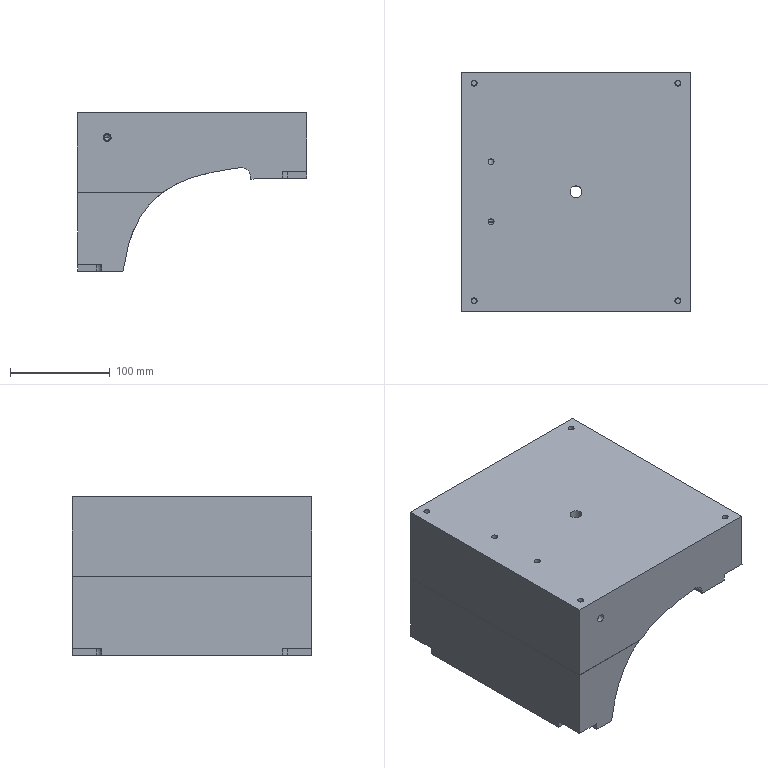Part | NX | features solid 2 | 1 solid | 145 faces | box 230 x 240 x 159.117 mm | volume 4798868 mm3 | spline 52 | plane 51 | cylinder 30 | sphere 6 | cone 6 | commonest cylinder face diameters 6 x15 8 x5 11 x4 20 x3 2 x2 12 x1